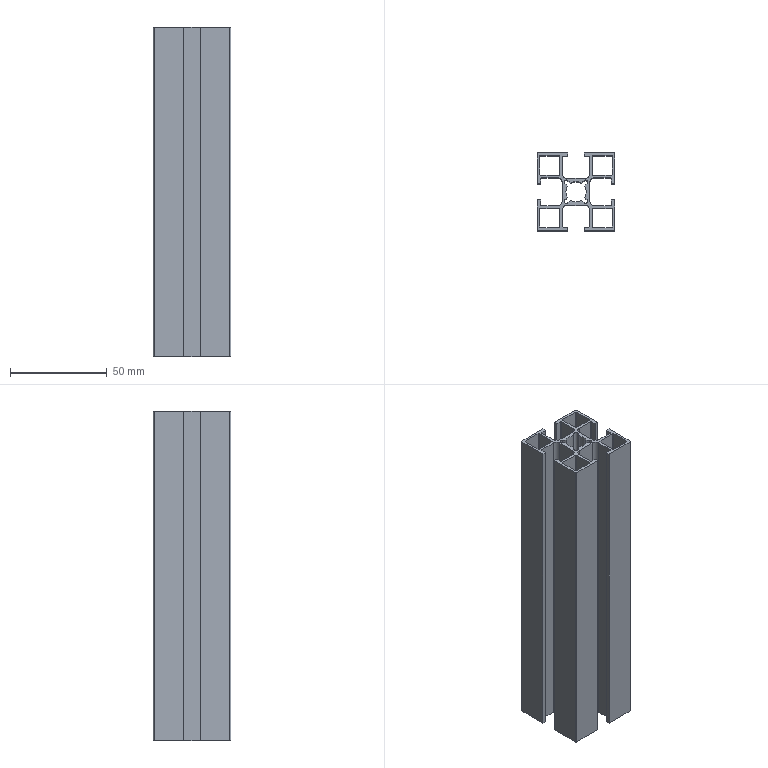Part | STEP file | GB4040-200 | 1 solid | 109 faces | box 40 x 40 x 170 mm | volume 64619 mm3 | plane 62 | cylinder 47 | commonest cylinder face diameters 1 x28 5 x8 2.2 x6 10.5 x5